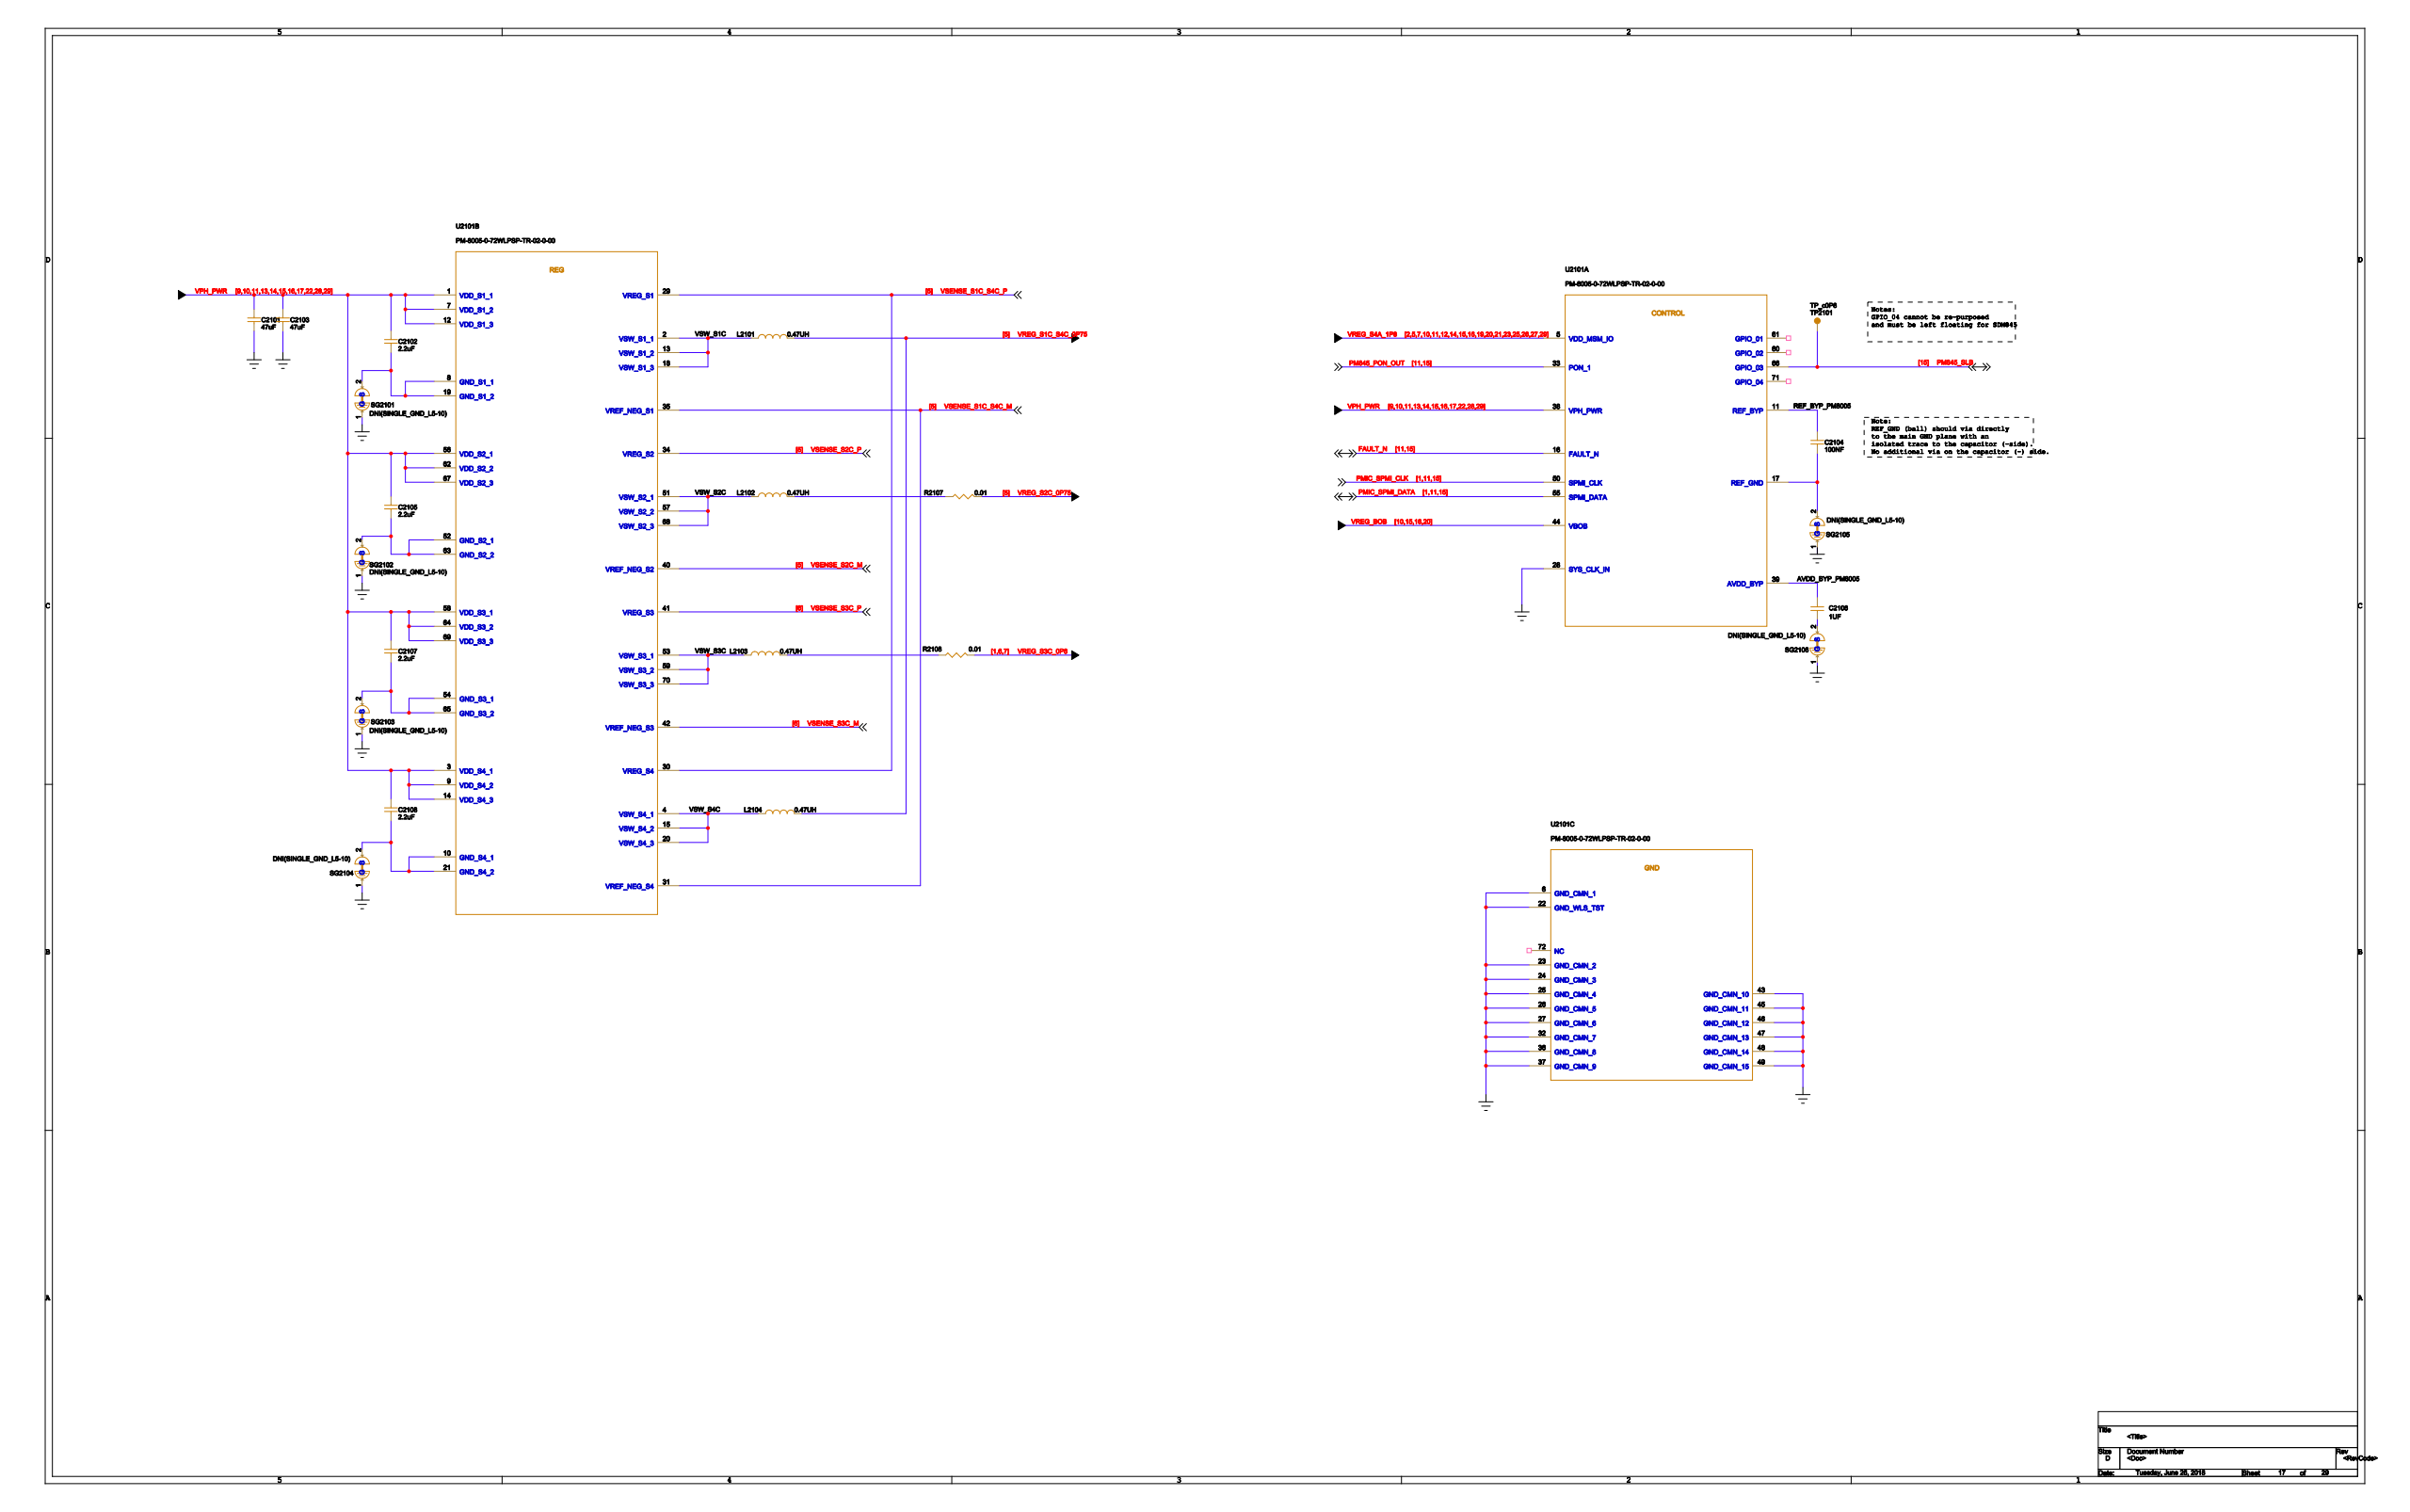Circuit board | Cadence Allegro | 802 parts | 566 nets | one sheet of the schematic
Parts on this sheet (reference | value | footprint):
C2101 | 47uF | C0805
C2102 | 2.2uF | 0402-BIG
C2103 | 47uF | C0805
C2104 | 100NF | C0201
C2105 | 2.2uF | 0402-BIG
C2106 | 1UF | C0402
C2107 | 2.2uF | 0402-BIG
C2108 | 2.2uF | 0402-BIG
L2101 | 0.47UH | L2016_MEKK2016
L2102 | 0.47UH | L2016_MEKK2016
L2103 | 0.47UH | L2016_MEKK2016
L2104 | 0.47UH | L2016_MEKK2016
R2107 | 0.01 | R0603
R2108 | 0.01 | R0603
SG2101 | DNI(SINGLE_GND_L5-10) | GND_L5-10
SG2102 | DNI(SINGLE_GND_L5-10) | GND_L5-10
SG2103 | DNI(SINGLE_GND_L5-10) | GND_L5-10
SG2104 | DNI(SINGLE_GND_L5-10) | GND_L5-10
SG2105 | DNI(SINGLE_GND_L5-10) | GND_L5-10
SG2106 | DNI(SINGLE_GND_L5-10) | GND_L5-10
TP2101 | TP_c0P6 | TP_C0P6
U2101 | PM-8005-0-72WLPSP-TR-02-0-00 | WLPSP72_2P82X3P44X0P63_0P35
Nets of these parts (net: part-pin ...):
GND: C2101-2 C2103-2 SG2101-1 SG2102-1 SG2103-1 SG2104-1 SG2105-1 SG2106-1 U2101-6 U2101-22 U2101-23 U2101-24 U2101-25 U2101-26 U2101-27 U2101-28 U2101-32 U2101-36 U2101-37 U2101-43 U2101-45 U2101-46 U2101-47 U2101-48 U2101-49
VPH_PWR: C2101-1 C2102-1 C2103-1 C2105-1 C2107-1 C2108-1 U2101-1 U2101-3 U2101-7 U2101-9 U2101-12 U2101-14 U2101-38 U2101-56 U2101-58 U2101-62 U2101-64 U2101-67 U2101-69
VREG_S4A_1P8: U2101-5
REF_BYP_PM8005: C2104-1 U2101-11
N263630: C2104-2 SG2105-2 U2101-17
VREG_S3C_0P6: R2108-2
VREG_BOB: U2101-44
VREG_S2C_0P75: R2107-2
N263068: L2103-2 R2108-1
N262074: L2102-2 R2107-1
VREG_S1C_S4C_0P75: L2101-2 L2104-2
N263060: C2106-1 SG2106-2
AVDD_BYP_PM8005: C2106-2 U2101-39
N263004: C2102-2 SG2101-2 U2101-8 U2101-19
N263016: C2105-2 SG2102-2 U2101-52 U2101-63
N263028: C2107-2 SG2103-2 U2101-54 U2101-65
N263040: C2108-2 SG2104-2 U2101-10 U2101-21
VSW_S1C: L2101-1 U2101-2 U2101-13 U2101-18
VSW_S2C: L2102-1 U2101-51 U2101-57 U2101-68
VSW_S3C: L2103-1 U2101-53 U2101-59 U2101-70
VSW_S4C: L2104-1 U2101-4 U2101-15 U2101-20
VSENSE_S2C_M: U2101-40
VSENSE_S1C_S4C_M: U2101-31 U2101-35
VSENSE_S2C_P: U2101-34
VSENSE_S1C_S4C_P: U2101-29 U2101-30
VSENSE_S3C_M: U2101-42
VSENSE_S3C_P: U2101-41
PM845_SLB: TP2101-1 U2101-66
PMIC_SPMI_DATA: U2101-55
PMIC_SPMI_CLK: U2101-50
PM845_PON_OUT: U2101-33
FAULT_N: U2101-16